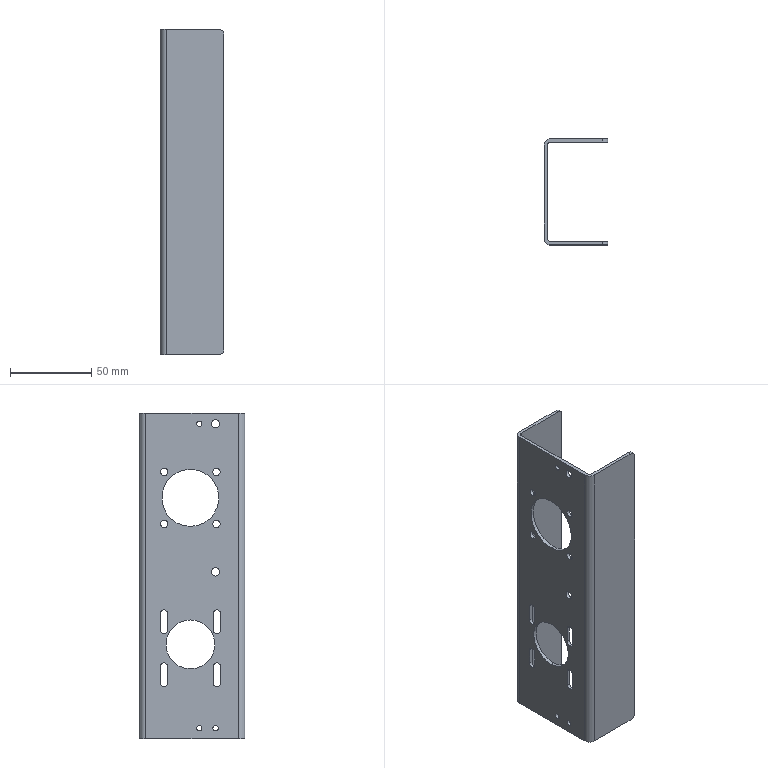Part | SolidWorks | features BaseBody 1 | 1 solid | 60 faces | box 39 x 65 x 200 mm | volume 50474 mm3 | cylinder 42 | plane 18 | commonest cylinder face diameters 4.5 x20 3.242 x6 5 x4 6 x4 4 x2 8 x2